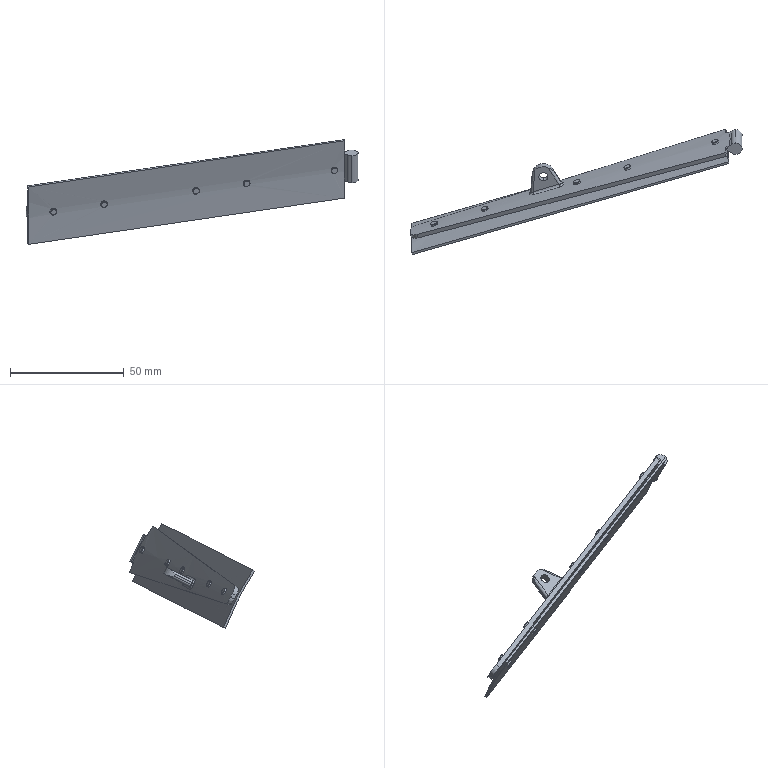Part | STEP file | Completa.sldasm-Part-148_Valor predeterminado | 1 solid | 106 faces | box 146.027 x 55.043 x 46.081 mm | volume 9453 mm3 | cylinder 45 | plane 23 | torus 20 | spline 15 | cone 3 | commonest cylinder face diameters 3 x30 1 x5 2 x4 5.5 x3 4 x2 10 x1